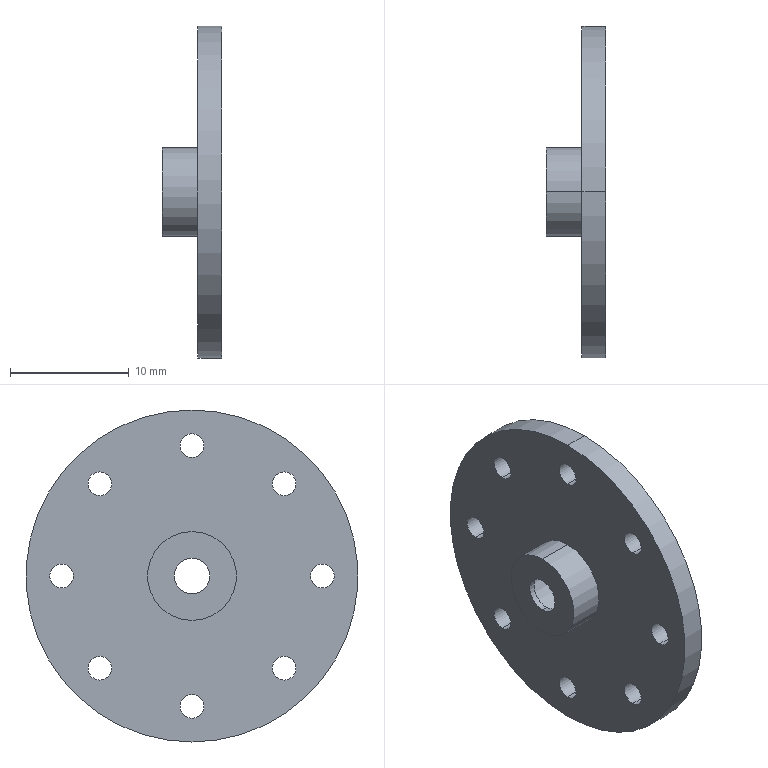Part | SolidWorks | features BaseBody 1 | 1 solid | 28 faces | box 5 x 28 x 28 mm | volume 1183 mm3 | cylinder 24 | plane 4 | commonest cylinder face diameters 2 x16 3 x2 6 x2 7.5 x2 28 x2
STEP:
#1=CARTESIAN_POINT('',(-2.,7.778,8.778));
#2=VERTEX_POINT('',#1);
#3=CARTESIAN_POINT('',(-2.,7.778,6.778));
#4=VERTEX_POINT('',#3);
#5=CARTESIAN_POINT('',(-2.,7.778,7.778));
#6=DIRECTION('',(1.,0.,0.));
#7=DIRECTION('',(0.,0.,-1.));
#8=AXIS2_PLACEMENT_3D('',#5,#6,#7);
#9=CIRCLE('',#8,1.);
#10=EDGE_CURVE('',#2,#4,#9,.T.);
#11=ORIENTED_EDGE('',*,*,#10,.F.);
#12=CARTESIAN_POINT('',(0.,7.778,8.778));
#13=VERTEX_POINT('',#12);
#14=CARTESIAN_POINT('',(-5.,7.778,8.778));
#15=DIRECTION('',(1.,0.,0.));
#16=VECTOR('',#15,1000.);
#17=LINE('',#14,#16);
#18=EDGE_CURVE('',#2,#13,#17,.T.);
#19=ORIENTED_EDGE('',*,*,#18,.T.);
#20=CARTESIAN_POINT('',(0.,7.778,6.778));
#21=VERTEX_POINT('',#20);
#22=CARTESIAN_POINT('',(0.,7.778,7.778));
#23=DIRECTION('',(1.,0.,0.));
#24=DIRECTION('',(0.,0.7071,-0.7071));
#25=AXIS2_PLACEMENT_3D('',#22,#23,#24);
#26=CIRCLE('',#25,1.);
#27=EDGE_CURVE('',#13,#21,#26,.T.);
#28=ORIENTED_EDGE('',*,*,#27,.T.);
#29=CARTESIAN_POINT('',(-5.,7.778,6.778));
#30=DIRECTION('',(1.,0.,0.));
#31=VECTOR('',#30,1000.);
#32=LINE('',#29,#31);
#33=EDGE_CURVE('',#4,#21,#32,.T.);
#34=ORIENTED_EDGE('',*,*,#33,.F.);
#35=EDGE_LOOP('',(#11,#19,#28,#34));
#36=FACE_OUTER_BOUND('',#35,.T.);
#37=CARTESIAN_POINT('',(-5.,7.778,7.778));
#38=DIRECTION('',(1.,0.,0.));
#39=DIRECTION('',(0.,0.,-1.));
#40=AXIS2_PLACEMENT_3D('',#37,#38,#39);
#41=CYLINDRICAL_SURFACE('',#40,1.);
#42=ADVANCED_FACE('',(#36),#41,.F.);
#43=CARTESIAN_POINT('',(-2.,0.,12.));
#44=VERTEX_POINT('',#43);
#45=CARTESIAN_POINT('',(-2.,0.,10.));
#46=VERTEX_POINT('',#45);
#47=CARTESIAN_POINT('',(-2.,0.,11.));
#48=DIRECTION('',(1.,0.,0.));
#49=DIRECTION('',(0.,0.,-1.));
#50=AXIS2_PLACEMENT_3D('',#47,#48,#49);
#51=CIRCLE('',#50,1.);
#52=EDGE_CURVE('',#44,#46,#51,.T.);
#53=ORIENTED_EDGE('',*,*,#52,.F.);
#54=CARTESIAN_POINT('',(0.,0.,12.));
#55=VERTEX_POINT('',#54);
#56=CARTESIAN_POINT('',(-5.,0.,12.));
#57=DIRECTION('',(1.,0.,0.));
#58=VECTOR('',#57,1000.);
#59=LINE('',#56,#58);
#60=EDGE_CURVE('',#44,#55,#59,.T.);
#61=ORIENTED_EDGE('',*,*,#60,.T.);
#62=CARTESIAN_POINT('',(0.,0.,10.));
#63=VERTEX_POINT('',#62);
#64=CARTESIAN_POINT('',(0.,0.,11.));
#65=DIRECTION('',(1.,0.,0.));
#66=DIRECTION('',(0.,1.,0.));
#67=AXIS2_PLACEMENT_3D('',#64,#65,#66);
#68=CIRCLE('',#67,1.);
#69=EDGE_CURVE('',#55,#63,#68,.T.);
#70=ORIENTED_EDGE('',*,*,#69,.T.);
#71=CARTESIAN_POINT('',(-5.,0.,10.));
#72=DIRECTION('',(1.,0.,0.));
#73=VECTOR('',#72,1000.);
#74=LINE('',#71,#73);
#75=EDGE_CURVE('',#46,#63,#74,.T.);
#76=ORIENTED_EDGE('',*,*,#75,.F.);
#77=EDGE_LOOP('',(#53,#61,#70,#76));
#78=FACE_OUTER_BOUND('',#77,.T.);
#79=CARTESIAN_POINT('',(-5.,0.,11.));
#80=DIRECTION('',(1.,0.,0.));
#81=DIRECTION('',(0.,0.,-1.));
#82=AXIS2_PLACEMENT_3D('',#79,#80,#81);
#83=CYLINDRICAL_SURFACE('',#82,1.);
#84=ADVANCED_FACE('',(#78),#83,.F.);
#85=CARTESIAN_POINT('',(-2.,-7.778,8.778));
#86=VERTEX_POINT('',#85);
#87=CARTESIAN_POINT('',(-2.,-7.778,6.778));
#88=VERTEX_POINT('',#87);
#89=CARTESIAN_POINT('',(-2.,-7.778,7.778));
#90=DIRECTION('',(1.,0.,0.));
#91=DIRECTION('',(0.,0.,-1.));
#92=AXIS2_PLACEMENT_3D('',#89,#90,#91);
#93=CIRCLE('',#92,1.);
#94=EDGE_CURVE('',#86,#88,#93,.T.);
#95=ORIENTED_EDGE('',*,*,#94,.F.);
#96=CARTESIAN_POINT('',(0.,-7.778,8.778));
#97=VERTEX_POINT('',#96);
#98=CARTESIAN_POINT('',(-5.,-7.778,8.778));
#99=DIRECTION('',(1.,0.,0.));
#100=VECTOR('',#99,1000.);
#101=LINE('',#98,#100);
#102=EDGE_CURVE('',#86,#97,#101,.T.);
#103=ORIENTED_EDGE('',*,*,#102,.T.);
#104=CARTESIAN_POINT('',(0.,-7.778,6.778));
#105=VERTEX_POINT('',#104);
#106=CARTESIAN_POINT('',(0.,-7.778,7.778));
#107=DIRECTION('',(1.,0.,0.));
#108=DIRECTION('',(0.,0.7071,0.7071));
#109=AXIS2_PLACEMENT_3D('',#106,#107,#108);
#110=CIRCLE('',#109,1.);
#111=EDGE_CURVE('',#97,#105,#110,.T.);
#112=ORIENTED_EDGE('',*,*,#111,.T.);
#113=CARTESIAN_POINT('',(-5.,-7.778,6.778));
#114=DIRECTION('',(1.,0.,0.));
#115=VECTOR('',#114,1000.);
#116=LINE('',#113,#115);
#117=EDGE_CURVE('',#88,#105,#116,.T.);
#118=ORIENTED_EDGE('',*,*,#117,.F.);
#119=EDGE_LOOP('',(#95,#103,#112,#118));
#120=FACE_OUTER_BOUND('',#119,.T.);
#121=CARTESIAN_POINT('',(-5.,-7.778,7.778));
#122=DIRECTION('',(1.,0.,0.));
#123=DIRECTION('',(0.,0.,-1.));
#124=AXIS2_PLACEMENT_3D('',#121,#122,#123);
#125=CYLINDRICAL_SURFACE('',#124,1.);
#126=ADVANCED_FACE('',(#120),#125,.F.);
#127=CARTESIAN_POINT('',(-2.,-11.,1.));
#128=VERTEX_POINT('',#127);
#129=CARTESIAN_POINT('',(-2.,-11.,-1.));
#130=VERTEX_POINT('',#129);
#131=CARTESIAN_POINT('',(-2.,-11.,0.));
#132=DIRECTION('',(1.,0.,0.));
#133=DIRECTION('',(0.,0.,-1.));
#134=AXIS2_PLACEMENT_3D('',#131,#132,#133);
#135=CIRCLE('',#134,1.);
#136=EDGE_CURVE('',#128,#130,#135,.T.);
#137=ORIENTED_EDGE('',*,*,#136,.F.);
#138=CARTESIAN_POINT('',(0.,-11.,1.));
#139=VERTEX_POINT('',#138);
#140=CARTESIAN_POINT('',(-5.,-11.,1.));
#141=DIRECTION('',(1.,0.,0.));
#142=VECTOR('',#141,1000.);
#143=LINE('',#140,#142);
#144=EDGE_CURVE('',#128,#139,#143,.T.);
#145=ORIENTED_EDGE('',*,*,#144,.T.);
#146=CARTESIAN_POINT('',(0.,-11.,-1.));
#147=VERTEX_POINT('',#146);
#148=CARTESIAN_POINT('',(0.,-11.,0.));
#149=DIRECTION('',(1.,0.,0.));
#150=DIRECTION('',(0.,0.,1.));
#151=AXIS2_PLACEMENT_3D('',#148,#149,#150);
#152=CIRCLE('',#151,1.);
#153=EDGE_CURVE('',#139,#147,#152,.T.);
#154=ORIENTED_EDGE('',*,*,#153,.T.);
#155=CARTESIAN_POINT('',(-5.,-11.,-1.));
#156=DIRECTION('',(1.,0.,0.));
#157=VECTOR('',#156,1000.);
#158=LINE('',#155,#157);
#159=EDGE_CURVE('',#130,#147,#158,.T.);
#160=ORIENTED_EDGE('',*,*,#159,.F.);
#161=EDGE_LOOP('',(#137,#145,#154,#160));
#162=FACE_OUTER_BOUND('',#161,.T.);
#163=CARTESIAN_POINT('',(-5.,-11.,0.));
#164=DIRECTION('',(1.,0.,0.));
#165=DIRECTION('',(0.,0.,-1.));
#166=AXIS2_PLACEMENT_3D('',#163,#164,#165);
#167=CYLINDRICAL_SURFACE('',#166,1.);
#168=ADVANCED_FACE('',(#162),#167,.F.);
#169=CARTESIAN_POINT('',(-2.,-7.778,-6.778));
#170=VERTEX_POINT('',#169);
#171=CARTESIAN_POINT('',(-2.,-7.778,-8.778));
#172=VERTEX_POINT('',#171);
#173=CARTESIAN_POINT('',(-2.,-7.778,-7.778));
#174=DIRECTION('',(1.,0.,0.));
#175=DIRECTION('',(0.,0.,-1.));
#176=AXIS2_PLACEMENT_3D('',#173,#174,#175);
#177=CIRCLE('',#176,1.);
#178=EDGE_CURVE('',#170,#172,#177,.T.);
#179=ORIENTED_EDGE('',*,*,#178,.F.);
#180=CARTESIAN_POINT('',(0.,-7.778,-6.778));
#181=VERTEX_POINT('',#180);
#182=CARTESIAN_POINT('',(-5.,-7.778,-6.778));
#183=DIRECTION('',(1.,0.,0.));
#184=VECTOR('',#183,1000.);
#185=LINE('',#182,#184);
#186=EDGE_CURVE('',#170,#181,#185,.T.);
#187=ORIENTED_EDGE('',*,*,#186,.T.);
#188=CARTESIAN_POINT('',(0.,-7.778,-8.778));
#189=VERTEX_POINT('',#188);
#190=CARTESIAN_POINT('',(0.,-7.778,-7.778));
#191=DIRECTION('',(1.,0.,0.));
#192=DIRECTION('',(0.,-0.7071,0.7071));
#193=AXIS2_PLACEMENT_3D('',#190,#191,#192);
#194=CIRCLE('',#193,1.);
#195=EDGE_CURVE('',#181,#189,#194,.T.);
#196=ORIENTED_EDGE('',*,*,#195,.T.);
#197=CARTESIAN_POINT('',(-5.,-7.778,-8.778));
#198=DIRECTION('',(1.,0.,0.));
#199=VECTOR('',#198,1000.);
#200=LINE('',#197,#199);
#201=EDGE_CURVE('',#172,#189,#200,.T.);
#202=ORIENTED_EDGE('',*,*,#201,.F.);
#203=EDGE_LOOP('',(#179,#187,#196,#202));
#204=FACE_OUTER_BOUND('',#203,.T.);
#205=CARTESIAN_POINT('',(-5.,-7.778,-7.778));
#206=DIRECTION('',(1.,0.,0.));
#207=DIRECTION('',(0.,0.,-1.));
#208=AXIS2_PLACEMENT_3D('',#205,#206,#207);
#209=CYLINDRICAL_SURFACE('',#208,1.);
#210=ADVANCED_FACE('',(#204),#209,.F.);
#211=CARTESIAN_POINT('',(-2.,0.,-10.));
#212=VERTEX_POINT('',#211);
#213=CARTESIAN_POINT('',(-2.,0.,-12.));
#214=VERTEX_POINT('',#213);
#215=CARTESIAN_POINT('',(-2.,0.,-11.));
#216=DIRECTION('',(1.,0.,0.));
#217=DIRECTION('',(0.,0.,-1.));
#218=AXIS2_PLACEMENT_3D('',#215,#216,#217);
#219=CIRCLE('',#218,1.);
#220=EDGE_CURVE('',#212,#214,#219,.T.);
#221=ORIENTED_EDGE('',*,*,#220,.F.);
#222=CARTESIAN_POINT('',(0.,0.,-10.));
#223=VERTEX_POINT('',#222);
#224=CARTESIAN_POINT('',(-5.,0.,-10.));
#225=DIRECTION('',(1.,0.,0.));
#226=VECTOR('',#225,1000.);
#227=LINE('',#224,#226);
#228=EDGE_CURVE('',#212,#223,#227,.T.);
#229=ORIENTED_EDGE('',*,*,#228,.T.);
#230=CARTESIAN_POINT('',(0.,0.,-12.));
#231=VERTEX_POINT('',#230);
#232=CARTESIAN_POINT('',(0.,0.,-11.));
#233=DIRECTION('',(1.,0.,0.));
#234=DIRECTION('',(0.,-1.,0.));
#235=AXIS2_PLACEMENT_3D('',#232,#233,#234);
#236=CIRCLE('',#235,1.);
#237=EDGE_CURVE('',#223,#231,#236,.T.);
#238=ORIENTED_EDGE('',*,*,#237,.T.);
#239=CARTESIAN_POINT('',(-5.,0.,-12.));
#240=DIRECTION('',(1.,0.,0.));
#241=VECTOR('',#240,1000.);
#242=LINE('',#239,#241);
#243=EDGE_CURVE('',#214,#231,#242,.T.);
#244=ORIENTED_EDGE('',*,*,#243,.F.);
#245=EDGE_LOOP('',(#221,#229,#238,#244));
#246=FACE_OUTER_BOUND('',#245,.T.);
#247=CARTESIAN_POINT('',(-5.,0.,-11.));
#248=DIRECTION('',(1.,0.,0.));
#249=DIRECTION('',(0.,0.,-1.));
#250=AXIS2_PLACEMENT_3D('',#247,#248,#249);
#251=CYLINDRICAL_SURFACE('',#250,1.);
#252=ADVANCED_FACE('',(#246),#251,.F.);
#253=CARTESIAN_POINT('',(-2.,7.778,-6.778));
#254=VERTEX_POINT('',#253);
#255=CARTESIAN_POINT('',(-2.,7.778,-8.778));
#256=VERTEX_POINT('',#255);
#257=CARTESIAN_POINT('',(-2.,7.778,-7.778));
#258=DIRECTION('',(1.,0.,0.));
#259=DIRECTION('',(0.,0.,-1.));
#260=AXIS2_PLACEMENT_3D('',#257,#258,#259);
#261=CIRCLE('',#260,1.);
#262=EDGE_CURVE('',#254,#256,#261,.T.);
#263=ORIENTED_EDGE('',*,*,#262,.F.);
#264=CARTESIAN_POINT('',(0.,7.778,-6.778));
#265=VERTEX_POINT('',#264);
#266=CARTESIAN_POINT('',(-5.,7.778,-6.778));
#267=DIRECTION('',(1.,0.,0.));
#268=VECTOR('',#267,1000.);
#269=LINE('',#266,#268);
#270=EDGE_CURVE('',#254,#265,#269,.T.);
#271=ORIENTED_EDGE('',*,*,#270,.T.);
#272=CARTESIAN_POINT('',(0.,7.778,-8.778));
#273=VERTEX_POINT('',#272);
#274=CARTESIAN_POINT('',(0.,7.778,-7.778));
#275=DIRECTION('',(1.,0.,0.));
#276=DIRECTION('',(0.,-0.7071,-0.7071));
#277=AXIS2_PLACEMENT_3D('',#274,#275,#276);
#278=CIRCLE('',#277,1.);
#279=EDGE_CURVE('',#265,#273,#278,.T.);
#280=ORIENTED_EDGE('',*,*,#279,.T.);
#281=CARTESIAN_POINT('',(-5.,7.778,-8.778));
#282=DIRECTION('',(1.,0.,0.));
#283=VECTOR('',#282,1000.);
#284=LINE('',#281,#283);
#285=EDGE_CURVE('',#256,#273,#284,.T.);
#286=ORIENTED_EDGE('',*,*,#285,.F.);
#287=EDGE_LOOP('',(#263,#271,#280,#286));
#288=FACE_OUTER_BOUND('',#287,.T.);
#289=CARTESIAN_POINT('',(-5.,7.778,-7.778));
#290=DIRECTION('',(1.,0.,0.));
#291=DIRECTION('',(0.,0.,-1.));
#292=AXIS2_PLACEMENT_3D('',#289,#290,#291);
#293=CYLINDRICAL_SURFACE('',#292,1.);
#294=ADVANCED_FACE('',(#288),#293,.F.);
#295=CARTESIAN_POINT('',(-2.,11.,1.));
#296=VERTEX_POINT('',#295);
#297=CARTESIAN_POINT('',(-2.,11.,-1.));
#298=VERTEX_POINT('',#297);
#299=CARTESIAN_POINT('',(-2.,11.,0.));
#300=DIRECTION('',(1.,0.,0.));
#301=DIRECTION('',(0.,0.,-1.));
#302=AXIS2_PLACEMENT_3D('',#299,#300,#301);
#303=CIRCLE('',#302,1.);
#304=EDGE_CURVE('',#296,#298,#303,.T.);
#305=ORIENTED_EDGE('',*,*,#304,.F.);
#306=CARTESIAN_POINT('',(0.,11.,1.));
#307=VERTEX_POINT('',#306);
#308=CARTESIAN_POINT('',(-5.,11.,1.));
#309=DIRECTION('',(1.,0.,0.));
#310=VECTOR('',#309,1000.);
#311=LINE('',#308,#310);
#312=EDGE_CURVE('',#296,#307,#311,.T.);
#313=ORIENTED_EDGE('',*,*,#312,.T.);
#314=CARTESIAN_POINT('',(0.,11.,-1.));
#315=VERTEX_POINT('',#314);
#316=CARTESIAN_POINT('',(0.,11.,0.));
#317=DIRECTION('',(1.,0.,0.));
#318=DIRECTION('',(0.,0.,-1.));
#319=AXIS2_PLACEMENT_3D('',#316,#317,#318);
#320=CIRCLE('',#319,1.);
#321=EDGE_CURVE('',#307,#315,#320,.T.);
#322=ORIENTED_EDGE('',*,*,#321,.T.);
#323=CARTESIAN_POINT('',(-5.,11.,-1.));
#324=DIRECTION('',(1.,0.,0.));
#325=VECTOR('',#324,1000.);
#326=LINE('',#323,#325);
#327=EDGE_CURVE('',#298,#315,#326,.T.);
#328=ORIENTED_EDGE('',*,*,#327,.F.);
#329=EDGE_LOOP('',(#305,#313,#322,#328));
#330=FACE_OUTER_BOUND('',#329,.T.);
#331=CARTESIAN_POINT('',(-5.,11.,0.));
#332=DIRECTION('',(1.,0.,0.));
#333=DIRECTION('',(0.,0.,-1.));
#334=AXIS2_PLACEMENT_3D('',#331,#332,#333);
#335=CYLINDRICAL_SURFACE('',#334,1.);
#336=ADVANCED_FACE('',(#330),#335,.F.);
#337=CARTESIAN_POINT('',(-4.5,0.,-1.5));
#338=VERTEX_POINT('',#337);
#339=CARTESIAN_POINT('',(-4.5,0.,1.5));
#340=VERTEX_POINT('',#339);
#341=CARTESIAN_POINT('',(-4.5,0.,0.));
#342=DIRECTION('',(-1.,0.,0.));
#343=DIRECTION('',(0.,0.,1.));
#344=AXIS2_PLACEMENT_3D('',#341,#342,#343);
#345=CIRCLE('',#344,1.5);
#346=EDGE_CURVE('',#338,#340,#345,.T.);
#347=ORIENTED_EDGE('',*,*,#346,.F.);
#348=CARTESIAN_POINT('',(-5.,0.,-1.5));
#349=VERTEX_POINT('',#348);
#350=CARTESIAN_POINT('',(0.,0.,-1.5));
#351=DIRECTION('',(-1.,0.,0.));
#352=VECTOR('',#351,1000.);
#353=LINE('',#350,#352);
#354=EDGE_CURVE('',#338,#349,#353,.T.);
#355=ORIENTED_EDGE('',*,*,#354,.T.);
#356=CARTESIAN_POINT('',(-5.,0.,1.5));
#357=VERTEX_POINT('',#356);
#358=CARTESIAN_POINT('',(-5.,0.,0.));
#359=DIRECTION('',(-1.,0.,0.));
#360=DIRECTION('',(0.,0.,1.));
#361=AXIS2_PLACEMENT_3D('',#358,#359,#360);
#362=CIRCLE('',#361,1.5);
#363=EDGE_CURVE('',#349,#357,#362,.T.);
#364=ORIENTED_EDGE('',*,*,#363,.T.);
#365=CARTESIAN_POINT('',(0.,0.,1.5));
#366=DIRECTION('',(-1.,0.,0.));
#367=VECTOR('',#366,1000.);
#368=LINE('',#365,#367);
#369=EDGE_CURVE('',#340,#357,#368,.T.);
#370=ORIENTED_EDGE('',*,*,#369,.F.);
#371=EDGE_LOOP('',(#347,#355,#364,#370));
#372=FACE_OUTER_BOUND('',#371,.T.);
#373=CARTESIAN_POINT('',(0.,0.,0.));
#374=DIRECTION('',(-1.,0.,0.));
#375=DIRECTION('',(0.,0.,1.));
#376=AXIS2_PLACEMENT_3D('',#373,#374,#375);
#377=CYLINDRICAL_SURFACE('',#376,1.5);
#378=ADVANCED_FACE('',(#372),#377,.F.);
#379=CARTESIAN_POINT('',(0.,0.,-3.));
#380=VERTEX_POINT('',#379);
#381=CARTESIAN_POINT('',(0.,0.,3.));
#382=VERTEX_POINT('',#381);
#383=CARTESIAN_POINT('',(0.,0.,0.));
#384=DIRECTION('',(-1.,0.,0.));
#385=DIRECTION('',(0.,0.,1.));
#386=AXIS2_PLACEMENT_3D('',#383,#384,#385);
#387=CIRCLE('',#386,3.);
#388=EDGE_CURVE('',#380,#382,#387,.T.);
#389=ORIENTED_EDGE('',*,*,#388,.F.);
#390=CARTESIAN_POINT('',(-4.5,0.,-3.));
#391=VERTEX_POINT('',#390);
#392=CARTESIAN_POINT('',(0.,0.,-3.));
#393=DIRECTION('',(-1.,0.,0.));
#394=VECTOR('',#393,1000.);
#395=LINE('',#392,#394);
#396=EDGE_CURVE('',#380,#391,#395,.T.);
#397=ORIENTED_EDGE('',*,*,#396,.T.);
#398=CARTESIAN_POINT('',(-4.5,0.,3.));
#399=VERTEX_POINT('',#398);
#400=CARTESIAN_POINT('',(-4.5,0.,0.));
#401=DIRECTION('',(-1.,0.,0.));
#402=DIRECTION('',(0.,0.,1.));
#403=AXIS2_PLACEMENT_3D('',#400,#401,#402);
#404=CIRCLE('',#403,3.);
#405=EDGE_CURVE('',#391,#399,#404,.T.);
#406=ORIENTED_EDGE('',*,*,#405,.T.);
#407=CARTESIAN_POINT('',(0.,0.,3.));
#408=DIRECTION('',(-1.,0.,0.));
#409=VECTOR('',#408,1000.);
#410=LINE('',#407,#409);
#411=EDGE_CURVE('',#382,#399,#410,.T.);
#412=ORIENTED_EDGE('',*,*,#411,.F.);
#413=EDGE_LOOP('',(#389,#397,#406,#412));
#414=FACE_OUTER_BOUND('',#413,.T.);
#415=CARTESIAN_POINT('',(0.,0.,0.));
#416=DIRECTION('',(-1.,0.,0.));
#417=DIRECTION('',(0.,0.,1.));
#418=AXIS2_PLACEMENT_3D('',#415,#416,#417);
#419=CYLINDRICAL_SURFACE('',#418,3.);
#420=ADVANCED_FACE('',(#414),#419,.F.);
#421=CARTESIAN_POINT('',(0.,0.,14.));
#422=VERTEX_POINT('',#421);
#423=CARTESIAN_POINT('',(0.,0.,-14.));
#424=VERTEX_POINT('',#423);
#425=CARTESIAN_POINT('',(0.,0.,0.));
#426=DIRECTION('',(-1.,0.,0.));
#427=DIRECTION('',(0.,0.,1.));
#428=AXIS2_PLACEMENT_3D('',#425,#426,#427);
#429=CIRCLE('',#428,14.);
#430=EDGE_CURVE('',#422,#424,#429,.T.);
#431=ORIENTED_EDGE('',*,*,#430,.T.);
#432=CARTESIAN_POINT('',(-2.,0.,-14.));
#433=VERTEX_POINT('',#432);
#434=CARTESIAN_POINT('',(0.,0.,-14.));
#435=DIRECTION('',(-1.,0.,0.));
#436=VECTOR('',#435,1000.);
#437=LINE('',#434,#436);
#438=EDGE_CURVE('',#424,#433,#437,.T.);
#439=ORIENTED_EDGE('',*,*,#438,.T.);
#440=CARTESIAN_POINT('',(-2.,0.,14.));
#441=VERTEX_POINT('',#440);
#442=CARTESIAN_POINT('',(-2.,0.,0.));
#443=DIRECTION('',(-1.,0.,0.));
#444=DIRECTION('',(0.,0.,1.));
#445=AXIS2_PLACEMENT_3D('',#442,#443,#444);
#446=CIRCLE('',#445,14.);
#447=EDGE_CURVE('',#441,#433,#446,.T.);
#448=ORIENTED_EDGE('',*,*,#447,.F.);
#449=CARTESIAN_POINT('',(0.,0.,14.));
#450=DIRECTION('',(-1.,0.,0.));
#451=VECTOR('',#450,1000.);
#452=LINE('',#449,#451);
#453=EDGE_CURVE('',#422,#441,#452,.T.);
#454=ORIENTED_EDGE('',*,*,#453,.F.);
#455=EDGE_LOOP('',(#431,#439,#448,#454));
#456=FACE_OUTER_BOUND('',#455,.T.);
#457=CARTESIAN_POINT('',(0.,0.,0.));
#458=DIRECTION('',(-1.,0.,0.));
#459=DIRECTION('',(0.,0.,1.));
#460=AXIS2_PLACEMENT_3D('',#457,#458,#459);
#461=CYLINDRICAL_SURFACE('',#460,14.);
#462=ADVANCED_FACE('',(#456),#461,.T.);
#463=CARTESIAN_POINT('',(-2.,0.,3.75));
#464=VERTEX_POINT('',#463);
#465=CARTESIAN_POINT('',(-2.,0.,-3.75));
#466=VERTEX_POINT('',#465);
#467=CARTESIAN_POINT('',(-2.,0.,0.));
#468=DIRECTION('',(-1.,0.,0.));
#469=DIRECTION('',(0.,0.,1.));
#470=AXIS2_PLACEMENT_3D('',#467,#468,#469);
#471=CIRCLE('',#470,3.75);
#472=EDGE_CURVE('',#464,#466,#471,.T.);
#473=ORIENTED_EDGE('',*,*,#472,.T.);
#474=CARTESIAN_POINT('',(-5.,0.,-3.75));
#475=VERTEX_POINT('',#474);
#476=CARTESIAN_POINT('',(0.,0.,-3.75));
#477=DIRECTION('',(-1.,0.,0.));
#478=VECTOR('',#477,1000.);
#479=LINE('',#476,#478);
#480=EDGE_CURVE('',#466,#475,#479,.T.);
#481=ORIENTED_EDGE('',*,*,#480,.T.);
#482=CARTESIAN_POINT('',(-5.,0.,3.75));
#483=VERTEX_POINT('',#482);
#484=CARTESIAN_POINT('',(-5.,0.,0.));
#485=DIRECTION('',(-1.,0.,0.));
#486=DIRECTION('',(0.,0.,1.));
#487=AXIS2_PLACEMENT_3D('',#484,#485,#486);
#488=CIRCLE('',#487,3.75);
#489=EDGE_CURVE('',#483,#475,#488,.T.);
#490=ORIENTED_EDGE('',*,*,#489,.F.);
#491=CARTESIAN_POINT('',(0.,0.,3.75));
#492=DIRECTION('',(-1.,0.,0.));
#493=VECTOR('',#492,1000.);
#494=LINE('',#491,#493);
#495=EDGE_CURVE('',#464,#483,#494,.T.);
#496=ORIENTED_EDGE('',*,*,#495,.F.);
#497=EDGE_LOOP('',(#473,#481,#490,#496));
#498=FACE_OUTER_BOUND('',#497,.T.);
#499=CARTESIAN_POINT('',(0.,0.,0.));
#500=DIRECTION('',(-1.,0.,0.));
#501=DIRECTION('',(0.,0.,1.));
#502=AXIS2_PLACEMENT_3D('',#499,#500,#501);
#503=CYLINDRICAL_SURFACE('',#502,3.75);
#504=ADVANCED_FACE('',(#498),#503,.T.);
#505=CARTESIAN_POINT('',(-5.,0.,0.));
#506=DIRECTION('',(-1.,0.,0.));
#507=DIRECTION('',(0.,0.,1.));
#508=AXIS2_PLACEMENT_3D('',#505,#506,#507);
#509=CIRCLE('',#508,1.5);
#510=EDGE_CURVE('',#357,#349,#509,.T.);
#511=ORIENTED_EDGE('',*,*,#510,.F.);
#512=ORIENTED_EDGE('',*,*,#363,.F.);
#513=EDGE_LOOP('',(#511,#512));
#514=FACE_BOUND('',#513,.T.);
#515=ORIENTED_EDGE('',*,*,#489,.T.);
#516=CARTESIAN_POINT('',(-5.,0.,0.));
#517=DIRECTION('',(-1.,0.,0.));
#518=DIRECTION('',(0.,0.,1.));
#519=AXIS2_PLACEMENT_3D('',#516,#517,#518);
#520=CIRCLE('',#519,3.75);
#521=EDGE_CURVE('',#475,#483,#520,.T.);
#522=ORIENTED_EDGE('',*,*,#521,.T.);
#523=EDGE_LOOP('',(#515,#522));
#524=FACE_OUTER_BOUND('',#523,.T.);
#525=CARTESIAN_POINT('',(-5.,1.5,0.));
#526=DIRECTION('',(1.,0.,0.));
#527=DIRECTION('',(0.,0.,-1.));
#528=AXIS2_PLACEMENT_3D('',#525,#526,#527);
#529=PLANE('',#528);
#530=ADVANCED_FACE('',(#514,#524),#529,.F.);
#531=ORIENTED_EDGE('',*,*,#480,.F.);
#532=CARTESIAN_POINT('',(-2.,0.,0.));
#533=DIRECTION('',(-1.,0.,0.));
#534=DIRECTION('',(0.,0.,1.));
#535=AXIS2_PLACEMENT_3D('',#532,#533,#534);
#536=CIRCLE('',#535,3.75);
#537=EDGE_CURVE('',#466,#464,#536,.T.);
#538=ORIENTED_EDGE('',*,*,#537,.T.);
#539=ORIENTED_EDGE('',*,*,#495,.T.);
#540=ORIENTED_EDGE('',*,*,#521,.F.);
#541=EDGE_LOOP('',(#531,#538,#539,#540));
#542=FACE_OUTER_BOUND('',#541,.T.);
#543=CARTESIAN_POINT('',(0.,0.,0.));
#544=DIRECTION('',(-1.,0.,0.));
#545=DIRECTION('',(0.,0.,1.));
#546=AXIS2_PLACEMENT_3D('',#543,#544,#545);
#547=CYLINDRICAL_SURFACE('',#546,3.75);
#548=ADVANCED_FACE('',(#542),#547,.T.);
#549=CARTESIAN_POINT('',(-2.,7.778,7.778));
#550=DIRECTION('',(1.,0.,0.));
#551=DIRECTION('',(0.,0.,-1.));
#552=AXIS2_PLACEMENT_3D('',#549,#550,#551);
#553=CIRCLE('',#552,1.);
#554=EDGE_CURVE('',#4,#2,#553,.T.);
#555=ORIENTED_EDGE('',*,*,#554,.T.);
#556=ORIENTED_EDGE('',*,*,#10,.T.);
#557=EDGE_LOOP('',(#555,#556));
#558=FACE_BOUND('',#557,.T.);
#559=CARTESIAN_POINT('',(-2.,0.,11.));
#560=DIRECTION('',(1.,0.,0.));
#561=DIRECTION('',(0.,0.,-1.));
#562=AXIS2_PLACEMENT_3D('',#559,#560,#561);
#563=CIRCLE('',#562,1.);
#564=EDGE_CURVE('',#46,#44,#563,.T.);
#565=ORIENTED_EDGE('',*,*,#564,.T.);
#566=ORIENTED_EDGE('',*,*,#52,.T.);
#567=EDGE_LOOP('',(#565,#566));
#568=FACE_BOUND('',#567,.T.);
#569=CARTESIAN_POINT('',(-2.,-7.778,7.778));
#570=DIRECTION('',(1.,0.,0.));
#571=DIRECTION('',(0.,0.,-1.));
#572=AXIS2_PLACEMENT_3D('',#569,#570,#571);
#573=CIRCLE('',#572,1.);
#574=EDGE_CURVE('',#88,#86,#573,.T.);
#575=ORIENTED_EDGE('',*,*,#574,.T.);
#576=ORIENTED_EDGE('',*,*,#94,.T.);
#577=EDGE_LOOP('',(#575,#576));
#578=FACE_BOUND('',#577,.T.);
#579=CARTESIAN_POINT('',(-2.,-11.,0.));
#580=DIRECTION('',(1.,0.,0.));
#581=DIRECTION('',(0.,0.,-1.));
#582=AXIS2_PLACEMENT_3D('',#579,#580,#581);
#583=CIRCLE('',#582,1.);
#584=EDGE_CURVE('',#130,#128,#583,.T.);
#585=ORIENTED_EDGE('',*,*,#584,.T.);
#586=ORIENTED_EDGE('',*,*,#136,.T.);
#587=EDGE_LOOP('',(#585,#586));
#588=FACE_BOUND('',#587,.T.);
#589=CARTESIAN_POINT('',(-2.,-7.778,-7.778));
#590=DIRECTION('',(1.,0.,0.));
#591=DIRECTION('',(0.,0.,-1.));
#592=AXIS2_PLACEMENT_3D('',#589,#590,#591);
#593=CIRCLE('',#592,1.);
#594=EDGE_CURVE('',#172,#170,#593,.T.);
#595=ORIENTED_EDGE('',*,*,#594,.T.);
#596=ORIENTED_EDGE('',*,*,#178,.T.);
#597=EDGE_LOOP('',(#595,#596));
#598=FACE_BOUND('',#597,.T.);
#599=CARTESIAN_POINT('',(-2.,0.,-11.));
#600=DIRECTION('',(1.,0.,0.));
#601=DIRECTION('',(0.,0.,-1.));
#602=AXIS2_PLACEMENT_3D('',#599,#600,#601);
#603=CIRCLE('',#602,1.);
#604=EDGE_CURVE('',#214,#212,#603,.T.);
#605=ORIENTED_EDGE('',*,*,#604,.T.);
#606=ORIENTED_EDGE('',*,*,#220,.T.);
#607=EDGE_LOOP('',(#605,#606));
#608=FACE_BOUND('',#607,.T.);
#609=CARTESIAN_POINT('',(-2.,7.778,-7.778));
#610=DIRECTION('',(1.,0.,0.));
#611=DIRECTION('',(0.,0.,-1.));
#612=AXIS2_PLACEMENT_3D('',#609,#610,#611);
#613=CIRCLE('',#612,1.);
#614=EDGE_CURVE('',#256,#254,#613,.T.);
#615=ORIENTED_EDGE('',*,*,#614,.T.);
#616=ORIENTED_EDGE('',*,*,#262,.T.);
#617=EDGE_LOOP('',(#615,#616));
#618=FACE_BOUND('',#617,.T.);
#619=CARTESIAN_POINT('',(-2.,11.,0.));
#620=DIRECTION('',(1.,0.,0.));
#621=DIRECTION('',(0.,0.,-1.));
#622=AXIS2_PLACEMENT_3D('',#619,#620,#621);
#623=CIRCLE('',#622,1.);
#624=EDGE_CURVE('',#298,#296,#623,.T.);
#625=ORIENTED_EDGE('',*,*,#624,.T.);
#626=ORIENTED_EDGE('',*,*,#304,.T.);
#627=EDGE_LOOP('',(#625,#626));
#628=FACE_BOUND('',#627,.T.);
#629=ORIENTED_EDGE('',*,*,#472,.F.);
#630=ORIENTED_EDGE('',*,*,#537,.F.);
#631=EDGE_LOOP('',(#629,#630));
#632=FACE_BOUND('',#631,.T.);
#633=ORIENTED_EDGE('',*,*,#447,.T.);
#634=CARTESIAN_POINT('',(-2.,0.,0.));
#635=DIRECTION('',(-1.,0.,0.));
#636=DIRECTION('',(0.,0.,1.));
#637=AXIS2_PLACEMENT_3D('',#634,#635,#636);
#638=CIRCLE('',#637,14.);
#639=EDGE_CURVE('',#433,#441,#638,.T.);
#640=ORIENTED_EDGE('',*,*,#639,.T.);
#641=EDGE_LOOP('',(#633,#640));
#642=FACE_OUTER_BOUND('',#641,.T.);
#643=CARTESIAN_POINT('',(-2.,3.75,0.));
#644=DIRECTION('',(1.,0.,0.));
#645=DIRECTION('',(0.,0.,-1.));
#646=AXIS2_PLACEMENT_3D('',#643,#644,#645);
#647=PLANE('',#646);
#648=ADVANCED_FACE('',(#558,#568,#578,#588,#598,#608,#618,#628,#632,#642),#647,.F.);
#649=ORIENTED_EDGE('',*,*,#438,.F.);
#650=CARTESIAN_POINT('',(0.,0.,0.));
#651=DIRECTION('',(-1.,0.,0.));
#652=DIRECTION('',(0.,0.,1.));
#653=AXIS2_PLACEMENT_3D('',#650,#651,#652);
#654=CIRCLE('',#653,14.);
#655=EDGE_CURVE('',#424,#422,#654,.T.);
#656=ORIENTED_EDGE('',*,*,#655,.T.);
#657=ORIENTED_EDGE('',*,*,#453,.T.);
#658=ORIENTED_EDGE('',*,*,#639,.F.);
#659=EDGE_LOOP('',(#649,#656,#657,#658));
#660=FACE_OUTER_BOUND('',#659,.T.);
#661=CARTESIAN_POINT('',(0.,0.,0.));
#662=DIRECTION('',(-1.,0.,0.));
#663=DIRECTION('',(0.,0.,1.));
#664=AXIS2_PLACEMENT_3D('',#661,#662,#663);
#665=CYLINDRICAL_SURFACE('',#664,14.);
#666=ADVANCED_FACE('',(#660),#665,.T.);
#667=CARTESIAN_POINT('',(0.,7.778,7.778));
#668=DIRECTION('',(1.,0.,0.));
#669=DIRECTION('',(0.,0.7071,-0.7071));
#670=AXIS2_PLACEMENT_3D('',#667,#668,#669);
#671=CIRCLE('',#670,1.);
#672=EDGE_CURVE('',#21,#13,#671,.T.);
#673=ORIENTED_EDGE('',*,*,#672,.F.);
#674=ORIENTED_EDGE('',*,*,#27,.F.);
#675=EDGE_LOOP('',(#673,#674));
#676=FACE_BOUND('',#675,.T.);
#677=CARTESIAN_POINT('',(0.,0.,11.));
#678=DIRECTION('',(1.,0.,0.));
#679=DIRECTION('',(0.,1.,0.));
#680=AXIS2_PLACEMENT_3D('',#677,#678,#679);
#681=CIRCLE('',#680,1.);
#682=EDGE_CURVE('',#63,#55,#681,.T.);
#683=ORIENTED_EDGE('',*,*,#682,.F.);
#684=ORIENTED_EDGE('',*,*,#69,.F.);
#685=EDGE_LOOP('',(#683,#684));
#686=FACE_BOUND('',#685,.T.);
#687=CARTESIAN_POINT('',(0.,-7.778,7.778));
#688=DIRECTION('',(1.,0.,0.));
#689=DIRECTION('',(0.,0.7071,0.7071));
#690=AXIS2_PLACEMENT_3D('',#687,#688,#689);
#691=CIRCLE('',#690,1.);
#692=EDGE_CURVE('',#105,#97,#691,.T.);
#693=ORIENTED_EDGE('',*,*,#692,.F.);
#694=ORIENTED_EDGE('',*,*,#111,.F.);
#695=EDGE_LOOP('',(#693,#694));
#696=FACE_BOUND('',#695,.T.);
#697=CARTESIAN_POINT('',(0.,-11.,0.));
#698=DIRECTION('',(1.,0.,0.));
#699=DIRECTION('',(0.,0.,1.));
#700=AXIS2_PLACEMENT_3D('',#697,#698,#699);
#701=CIRCLE('',#700,1.);
#702=EDGE_CURVE('',#147,#139,#701,.T.);
#703=ORIENTED_EDGE('',*,*,#702,.F.);
#704=ORIENTED_EDGE('',*,*,#153,.F.);
#705=EDGE_LOOP('',(#703,#704));
#706=FACE_BOUND('',#705,.T.);
#707=CARTESIAN_POINT('',(0.,-7.778,-7.778));
#708=DIRECTION('',(1.,0.,0.));
#709=DIRECTION('',(0.,-0.7071,0.7071));
#710=AXIS2_PLACEMENT_3D('',#707,#708,#709);
#711=CIRCLE('',#710,1.);
#712=EDGE_CURVE('',#189,#181,#711,.T.);
#713=ORIENTED_EDGE('',*,*,#712,.F.);
#714=ORIENTED_EDGE('',*,*,#195,.F.);
#715=EDGE_LOOP('',(#713,#714));
#716=FACE_BOUND('',#715,.T.);
#717=CARTESIAN_POINT('',(0.,0.,-11.));
#718=DIRECTION('',(1.,0.,0.));
#719=DIRECTION('',(0.,-1.,0.));
#720=AXIS2_PLACEMENT_3D('',#717,#718,#719);
#721=CIRCLE('',#720,1.);
#722=EDGE_CURVE('',#231,#223,#721,.T.);
#723=ORIENTED_EDGE('',*,*,#722,.F.);
#724=ORIENTED_EDGE('',*,*,#237,.F.);
#725=EDGE_LOOP('',(#723,#724));
#726=FACE_BOUND('',#725,.T.);
#727=CARTESIAN_POINT('',(0.,7.778,-7.778));
#728=DIRECTION('',(1.,0.,0.));
#729=DIRECTION('',(0.,-0.7071,-0.7071));
#730=AXIS2_PLACEMENT_3D('',#727,#728,#729);
#731=CIRCLE('',#730,1.);
#732=EDGE_CURVE('',#273,#265,#731,.T.);
#733=ORIENTED_EDGE('',*,*,#732,.F.);
#734=ORIENTED_EDGE('',*,*,#279,.F.);
#735=EDGE_LOOP('',(#733,#734));
#736=FACE_BOUND('',#735,.T.);
#737=CARTESIAN_POINT('',(0.,11.,0.));
#738=DIRECTION('',(1.,0.,0.));
#739=DIRECTION('',(0.,0.,-1.));
#740=AXIS2_PLACEMENT_3D('',#737,#738,#739);
#741=CIRCLE('',#740,1.);
#742=EDGE_CURVE('',#315,#307,#741,.T.);
#743=ORIENTED_EDGE('',*,*,#742,.F.);
#744=ORIENTED_EDGE('',*,*,#321,.F.);
#745=EDGE_LOOP('',(#743,#744));
#746=FACE_BOUND('',#745,.T.);
#747=ORIENTED_EDGE('',*,*,#430,.F.);
#748=ORIENTED_EDGE('',*,*,#655,.F.);
#749=EDGE_LOOP('',(#747,#748));
#750=FACE_OUTER_BOUND('',#749,.T.);
#751=CARTESIAN_POINT('',(0.,0.,0.));
#752=DIRECTION('',(-1.,0.,0.));
#753=DIRECTION('',(0.,0.,1.));
#754=AXIS2_PLACEMENT_3D('',#751,#752,#753);
#755=CIRCLE('',#754,3.);
#756=EDGE_CURVE('',#382,#380,#755,.T.);
#757=ORIENTED_EDGE('',*,*,#756,.T.);
#758=ORIENTED_EDGE('',*,*,#388,.T.);
#759=EDGE_LOOP('',(#757,#758));
#760=FACE_BOUND('',#759,.T.);
#761=CARTESIAN_POINT('',(0.,14.,0.));
#762=DIRECTION('',(-1.,0.,0.));
#763=DIRECTION('',(0.,0.,1.));
#764=AXIS2_PLACEMENT_3D('',#761,#762,#763);
#765=PLANE('',#764);
#766=ADVANCED_FACE('',(#676,#686,#696,#706,#716,#726,#736,#746,#750,#760),#765,.F.);
#767=ORIENTED_EDGE('',*,*,#396,.F.);
#768=ORIENTED_EDGE('',*,*,#756,.F.);
#769=ORIENTED_EDGE('',*,*,#411,.T.);
#770=CARTESIAN_POINT('',(-4.5,0.,0.));
#771=DIRECTION('',(-1.,0.,0.));
#772=DIRECTION('',(0.,0.,1.));
#773=AXIS2_PLACEMENT_3D('',#770,#771,#772);
#774=CIRCLE('',#773,3.);
#775=EDGE_CURVE('',#399,#391,#774,.T.);
#776=ORIENTED_EDGE('',*,*,#775,.T.);
#777=EDGE_LOOP('',(#767,#768,#769,#776));
#778=FACE_OUTER_BOUND('',#777,.T.);
#779=CARTESIAN_POINT('',(0.,0.,0.));
#780=DIRECTION('',(-1.,0.,0.));
#781=DIRECTION('',(0.,0.,1.));
#782=AXIS2_PLACEMENT_3D('',#779,#780,#781);
#783=CYLINDRICAL_SURFACE('',#782,3.);
#784=ADVANCED_FACE('',(#778),#783,.F.);
#785=ORIENTED_EDGE('',*,*,#775,.F.);
#786=ORIENTED_EDGE('',*,*,#405,.F.);
#787=EDGE_LOOP('',(#785,#786));
#788=FACE_OUTER_BOUND('',#787,.T.);
#789=CARTESIAN_POINT('',(-4.5,0.,0.));
#790=DIRECTION('',(-1.,0.,0.));
#791=DIRECTION('',(0.,0.,1.));
#792=AXIS2_PLACEMENT_3D('',#789,#790,#791);
#793=CIRCLE('',#792,1.5);
#794=EDGE_CURVE('',#340,#338,#793,.T.);
#795=ORIENTED_EDGE('',*,*,#794,.T.);
#796=ORIENTED_EDGE('',*,*,#346,.T.);
#797=EDGE_LOOP('',(#795,#796));
#798=FACE_BOUND('',#797,.T.);
#799=CARTESIAN_POINT('',(-4.5,3.,0.));
#800=DIRECTION('',(-1.,0.,0.));
#801=DIRECTION('',(0.,0.,1.));
#802=AXIS2_PLACEMENT_3D('',#799,#800,#801);
#803=PLANE('',#802);
#804=ADVANCED_FACE('',(#788,#798),#803,.F.);
#805=ORIENTED_EDGE('',*,*,#354,.F.);
#806=ORIENTED_EDGE('',*,*,#794,.F.);
#807=ORIENTED_EDGE('',*,*,#369,.T.);
#808=ORIENTED_EDGE('',*,*,#510,.T.);
#809=EDGE_LOOP('',(#805,#806,#807,#808));
#810=FACE_OUTER_BOUND('',#809,.T.);
#811=CARTESIAN_POINT('',(0.,0.,0.));
#812=DIRECTION('',(-1.,0.,0.));
#813=DIRECTION('',(0.,0.,1.));
#814=AXIS2_PLACEMENT_3D('',#811,#812,#813);
#815=CYLINDRICAL_SURFACE('',#814,1.5);
#816=ADVANCED_FACE('',(#810),#815,.F.);
#817=ORIENTED_EDGE('',*,*,#312,.F.);
#818=ORIENTED_EDGE('',*,*,#624,.F.);
#819=ORIENTED_EDGE('',*,*,#327,.T.);
#820=ORIENTED_EDGE('',*,*,#742,.T.);
#821=EDGE_LOOP('',(#817,#818,#819,#820));
#822=FACE_OUTER_BOUND('',#821,.T.);
#823=CARTESIAN_POINT('',(-5.,11.,0.));
#824=DIRECTION('',(1.,0.,0.));
#825=DIRECTION('',(0.,0.,-1.));
#826=AXIS2_PLACEMENT_3D('',#823,#824,#825);
#827=CYLINDRICAL_SURFACE('',#826,1.);
#828=ADVANCED_FACE('',(#822),#827,.F.);
#829=ORIENTED_EDGE('',*,*,#270,.F.);
#830=ORIENTED_EDGE('',*,*,#614,.F.);
#831=ORIENTED_EDGE('',*,*,#285,.T.);
#832=ORIENTED_EDGE('',*,*,#732,.T.);
#833=EDGE_LOOP('',(#829,#830,#831,#832));
#834=FACE_OUTER_BOUND('',#833,.T.);
#835=CARTESIAN_POINT('',(-5.,7.778,-7.778));
#836=DIRECTION('',(1.,0.,0.));
#837=DIRECTION('',(0.,0.,-1.));
#838=AXIS2_PLACEMENT_3D('',#835,#836,#837);
#839=CYLINDRICAL_SURFACE('',#838,1.);
#840=ADVANCED_FACE('',(#834),#839,.F.);
#841=ORIENTED_EDGE('',*,*,#228,.F.);
#842=ORIENTED_EDGE('',*,*,#604,.F.);
#843=ORIENTED_EDGE('',*,*,#243,.T.);
#844=ORIENTED_EDGE('',*,*,#722,.T.);
#845=EDGE_LOOP('',(#841,#842,#843,#844));
#846=FACE_OUTER_BOUND('',#845,.T.);
#847=CARTESIAN_POINT('',(-5.,0.,-11.));
#848=DIRECTION('',(1.,0.,0.));
#849=DIRECTION('',(0.,0.,-1.));
#850=AXIS2_PLACEMENT_3D('',#847,#848,#849);
#851=CYLINDRICAL_SURFACE('',#850,1.);
#852=ADVANCED_FACE('',(#846),#851,.F.);
#853=ORIENTED_EDGE('',*,*,#186,.F.);
#854=ORIENTED_EDGE('',*,*,#594,.F.);
#855=ORIENTED_EDGE('',*,*,#201,.T.);
#856=ORIENTED_EDGE('',*,*,#712,.T.);
#857=EDGE_LOOP('',(#853,#854,#855,#856));
#858=FACE_OUTER_BOUND('',#857,.T.);
#859=CARTESIAN_POINT('',(-5.,-7.778,-7.778));
#860=DIRECTION('',(1.,0.,0.));
#861=DIRECTION('',(0.,0.,-1.));
#862=AXIS2_PLACEMENT_3D('',#859,#860,#861);
#863=CYLINDRICAL_SURFACE('',#862,1.);
#864=ADVANCED_FACE('',(#858),#863,.F.);
#865=ORIENTED_EDGE('',*,*,#144,.F.);
#866=ORIENTED_EDGE('',*,*,#584,.F.);
#867=ORIENTED_EDGE('',*,*,#159,.T.);
#868=ORIENTED_EDGE('',*,*,#702,.T.);
#869=EDGE_LOOP('',(#865,#866,#867,#868));
#870=FACE_OUTER_BOUND('',#869,.T.);
#871=CARTESIAN_POINT('',(-5.,-11.,0.));
#872=DIRECTION('',(1.,0.,0.));
#873=DIRECTION('',(0.,0.,-1.));
#874=AXIS2_PLACEMENT_3D('',#871,#872,#873);
#875=CYLINDRICAL_SURFACE('',#874,1.);
#876=ADVANCED_FACE('',(#870),#875,.F.);
#877=ORIENTED_EDGE('',*,*,#102,.F.);
#878=ORIENTED_EDGE('',*,*,#574,.F.);
#879=ORIENTED_EDGE('',*,*,#117,.T.);
#880=ORIENTED_EDGE('',*,*,#692,.T.);
#881=EDGE_LOOP('',(#877,#878,#879,#880));
#882=FACE_OUTER_BOUND('',#881,.T.);
#883=CARTESIAN_POINT('',(-5.,-7.778,7.778));
#884=DIRECTION('',(1.,0.,0.));
#885=DIRECTION('',(0.,0.,-1.));
#886=AXIS2_PLACEMENT_3D('',#883,#884,#885);
#887=CYLINDRICAL_SURFACE('',#886,1.);
#888=ADVANCED_FACE('',(#882),#887,.F.);
#889=ORIENTED_EDGE('',*,*,#60,.F.);
#890=ORIENTED_EDGE('',*,*,#564,.F.);
#891=ORIENTED_EDGE('',*,*,#75,.T.);
#892=ORIENTED_EDGE('',*,*,#682,.T.);
#893=EDGE_LOOP('',(#889,#890,#891,#892));
#894=FACE_OUTER_BOUND('',#893,.T.);
#895=CARTESIAN_POINT('',(-5.,0.,11.));
#896=DIRECTION('',(1.,0.,0.));
#897=DIRECTION('',(0.,0.,-1.));
#898=AXIS2_PLACEMENT_3D('',#895,#896,#897);
#899=CYLINDRICAL_SURFACE('',#898,1.);
#900=ADVANCED_FACE('',(#894),#899,.F.);
#901=ORIENTED_EDGE('',*,*,#18,.F.);
#902=ORIENTED_EDGE('',*,*,#554,.F.);
#903=ORIENTED_EDGE('',*,*,#33,.T.);
#904=ORIENTED_EDGE('',*,*,#672,.T.);
#905=EDGE_LOOP('',(#901,#902,#903,#904));
#906=FACE_OUTER_BOUND('',#905,.T.);
#907=CARTESIAN_POINT('',(-5.,7.778,7.778));
#908=DIRECTION('',(1.,0.,0.));
#909=DIRECTION('',(0.,0.,-1.));
#910=AXIS2_PLACEMENT_3D('',#907,#908,#909);
#911=CYLINDRICAL_SURFACE('',#910,1.);
#912=ADVANCED_FACE('',(#906),#911,.F.);
#913=CLOSED_SHELL('',(#42,#84,#126,#168,#210,#252,#294,#336,#378,#420,#462,#504,#530,#548,#648,#666,#766,#784,#804,#816,#828,#840,#852,#864,#876,#888,#900,#912));
#914=MANIFOLD_SOLID_BREP('',#913);
#915=CARTESIAN_POINT('',(0.,0.,0.));
#916=DIRECTION('',(0.,0.,1.));
#917=DIRECTION('',(1.,0.,0.));
#918=AXIS2_PLACEMENT_3D('',#915,#916,#917);
#919=(LENGTH_UNIT()NAMED_UNIT(*)SI_UNIT(.MILLI.,.METRE.));
#920=UNCERTAINTY_MEASURE_WITH_UNIT(LENGTH_MEASURE(0.00001),#919,'','');
#921=(NAMED_UNIT(*)PLANE_ANGLE_UNIT()SI_UNIT($,.RADIAN.));
#922=(NAMED_UNIT(*)SI_UNIT($,.STERADIAN.)SOLID_ANGLE_UNIT());
#923=(GEOMETRIC_REPRESENTATION_CONTEXT(3)GLOBAL_UNCERTAINTY_ASSIGNED_CONTEXT((#920))GLOBAL_UNIT_ASSIGNED_CONTEXT((#919,#921,#922))REPRESENTATION_CONTEXT('',''));
#924=ADVANCED_BREP_SHAPE_REPRESENTATION('',(#914,#918),#923);